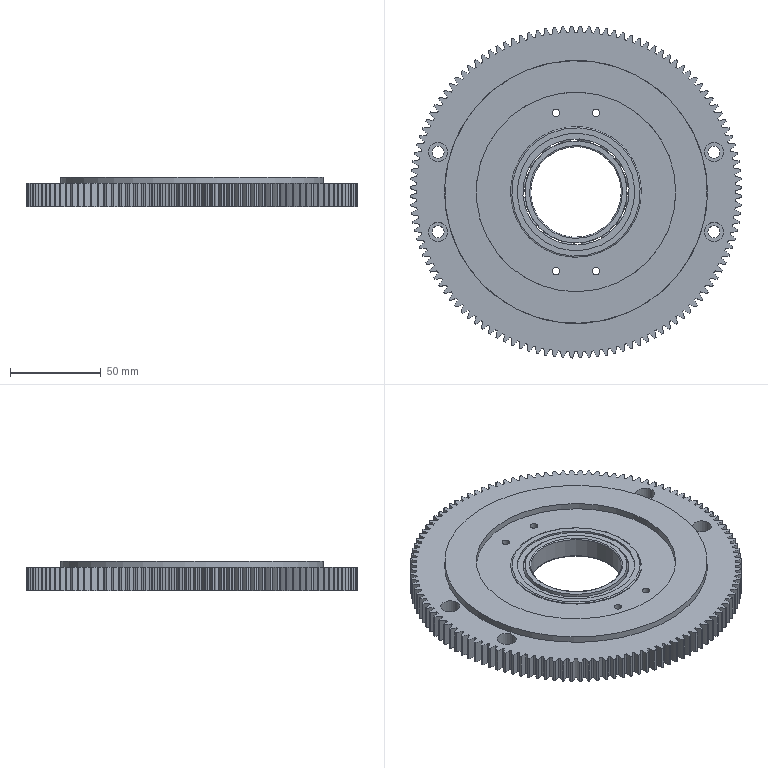Part | NX | features BREP 3 | 3 solids | 673 faces | box 182.961 x 182.961 x 16.5 mm | volume 312056 mm3 | cylinder 518 | sphere 64 | plane 55 | torus 36 | commonest cylinder face diameters 72 x242 176.248 x120 183 x120 6.6 x8 10.5 x8 4.2 x4